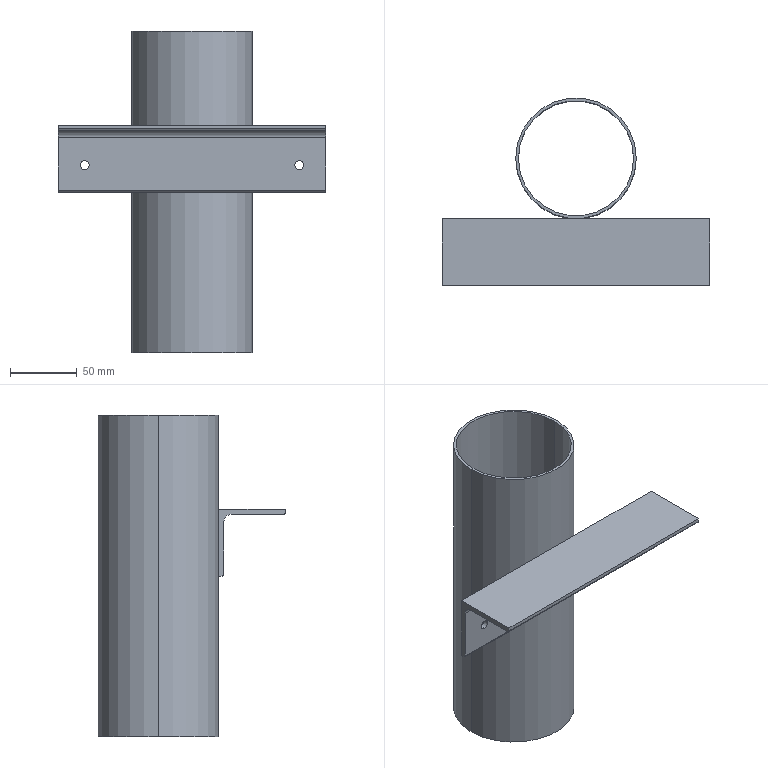Part | SolidWorks | features 3DProfileFeature 1, HoleWzd 1, ICE 1, WeldMemberFeat 1, WeldmentFeature 1 | 2 solids | 21 faces | box 200 x 140 x 240 mm | volume 210373 mm3 | cylinder 11 | plane 10 | commonest cylinder face diameters 6.6 x4 2.667 x2 86 x2 90 x2 11 x1
STEP:
#1=CARTESIAN_POINT('',(143.,45.,70.));
#2=VERTEX_POINT('',#1);
#3=CARTESIAN_POINT('',(57.,45.,70.));
#4=VERTEX_POINT('',#3);
#5=CARTESIAN_POINT('',(100.,45.,70.));
#6=DIRECTION('',(0.,0.,-1.));
#7=DIRECTION('',(-1.,0.,0.));
#8=AXIS2_PLACEMENT_3D('',#5,#6,#7);
#9=CIRCLE('',#8,43.);
#10=EDGE_CURVE('',#2,#4,#9,.T.);
#11=ORIENTED_EDGE('',*,*,#10,.F.);
#12=CARTESIAN_POINT('',(143.,45.,-170.));
#13=VERTEX_POINT('',#12);
#14=CARTESIAN_POINT('',(143.,45.,70.));
#15=DIRECTION('',(0.,0.,-1.));
#16=VECTOR('',#15,1000.);
#17=LINE('',#14,#16);
#18=EDGE_CURVE('',#2,#13,#17,.T.);
#19=ORIENTED_EDGE('',*,*,#18,.T.);
#20=CARTESIAN_POINT('',(57.,45.,-170.));
#21=VERTEX_POINT('',#20);
#22=CARTESIAN_POINT('',(100.,45.,-170.));
#23=DIRECTION('',(0.,0.,-1.));
#24=DIRECTION('',(-1.,0.,0.));
#25=AXIS2_PLACEMENT_3D('',#22,#23,#24);
#26=CIRCLE('',#25,43.);
#27=EDGE_CURVE('',#13,#21,#26,.T.);
#28=ORIENTED_EDGE('',*,*,#27,.T.);
#29=CARTESIAN_POINT('',(57.,45.,70.));
#30=DIRECTION('',(0.,0.,-1.));
#31=VECTOR('',#30,1000.);
#32=LINE('',#29,#31);
#33=EDGE_CURVE('',#4,#21,#32,.T.);
#34=ORIENTED_EDGE('',*,*,#33,.F.);
#35=EDGE_LOOP('',(#11,#19,#28,#34));
#36=FACE_OUTER_BOUND('',#35,.T.);
#37=CARTESIAN_POINT('',(100.,45.,70.));
#38=DIRECTION('',(0.,0.,-1.));
#39=DIRECTION('',(-1.,0.,0.));
#40=AXIS2_PLACEMENT_3D('',#37,#38,#39);
#41=CYLINDRICAL_SURFACE('',#40,43.);
#42=ADVANCED_FACE('',(#36),#41,.F.);
#43=CARTESIAN_POINT('',(55.,45.,70.));
#44=VERTEX_POINT('',#43);
#45=CARTESIAN_POINT('',(145.,45.,70.));
#46=VERTEX_POINT('',#45);
#47=CARTESIAN_POINT('',(100.,45.,70.));
#48=DIRECTION('',(0.,0.,-1.));
#49=DIRECTION('',(-1.,0.,0.));
#50=AXIS2_PLACEMENT_3D('',#47,#48,#49);
#51=CIRCLE('',#50,45.);
#52=EDGE_CURVE('',#44,#46,#51,.T.);
#53=ORIENTED_EDGE('',*,*,#52,.T.);
#54=CARTESIAN_POINT('',(145.,45.,-170.));
#55=VERTEX_POINT('',#54);
#56=CARTESIAN_POINT('',(145.,45.,70.));
#57=DIRECTION('',(0.,0.,-1.));
#58=VECTOR('',#57,1000.);
#59=LINE('',#56,#58);
#60=EDGE_CURVE('',#46,#55,#59,.T.);
#61=ORIENTED_EDGE('',*,*,#60,.T.);
#62=CARTESIAN_POINT('',(55.,45.,-170.));
#63=VERTEX_POINT('',#62);
#64=CARTESIAN_POINT('',(100.,45.,-170.));
#65=DIRECTION('',(0.,0.,-1.));
#66=DIRECTION('',(-1.,0.,0.));
#67=AXIS2_PLACEMENT_3D('',#64,#65,#66);
#68=CIRCLE('',#67,45.);
#69=EDGE_CURVE('',#63,#55,#68,.T.);
#70=ORIENTED_EDGE('',*,*,#69,.F.);
#71=CARTESIAN_POINT('',(55.,45.,70.));
#72=DIRECTION('',(0.,0.,-1.));
#73=VECTOR('',#72,1000.);
#74=LINE('',#71,#73);
#75=EDGE_CURVE('',#44,#63,#74,.T.);
#76=ORIENTED_EDGE('',*,*,#75,.F.);
#77=EDGE_LOOP('',(#53,#61,#70,#76));
#78=FACE_OUTER_BOUND('',#77,.T.);
#79=CARTESIAN_POINT('',(100.,45.,70.));
#80=DIRECTION('',(0.,0.,-1.));
#81=DIRECTION('',(-1.,0.,0.));
#82=AXIS2_PLACEMENT_3D('',#79,#80,#81);
#83=CYLINDRICAL_SURFACE('',#82,45.);
#84=ADVANCED_FACE('',(#78),#83,.T.);
#85=ORIENTED_EDGE('',*,*,#60,.F.);
#86=CARTESIAN_POINT('',(100.,45.,70.));
#87=DIRECTION('',(0.,0.,-1.));
#88=DIRECTION('',(-1.,0.,0.));
#89=AXIS2_PLACEMENT_3D('',#86,#87,#88);
#90=CIRCLE('',#89,45.);
#91=EDGE_CURVE('',#46,#44,#90,.T.);
#92=ORIENTED_EDGE('',*,*,#91,.T.);
#93=ORIENTED_EDGE('',*,*,#75,.T.);
#94=CARTESIAN_POINT('',(100.,45.,-170.));
#95=DIRECTION('',(0.,0.,-1.));
#96=DIRECTION('',(-1.,0.,0.));
#97=AXIS2_PLACEMENT_3D('',#94,#95,#96);
#98=CIRCLE('',#97,45.);
#99=EDGE_CURVE('',#55,#63,#98,.T.);
#100=ORIENTED_EDGE('',*,*,#99,.F.);
#101=EDGE_LOOP('',(#85,#92,#93,#100));
#102=FACE_OUTER_BOUND('',#101,.T.);
#103=CARTESIAN_POINT('',(100.,45.,70.));
#104=DIRECTION('',(0.,0.,-1.));
#105=DIRECTION('',(-1.,0.,0.));
#106=AXIS2_PLACEMENT_3D('',#103,#104,#105);
#107=CYLINDRICAL_SURFACE('',#106,45.);
#108=ADVANCED_FACE('',(#102),#107,.T.);
#109=CARTESIAN_POINT('',(100.,45.,70.));
#110=DIRECTION('',(0.,0.,-1.));
#111=DIRECTION('',(-1.,0.,0.));
#112=AXIS2_PLACEMENT_3D('',#109,#110,#111);
#113=CIRCLE('',#112,43.);
#114=EDGE_CURVE('',#4,#2,#113,.T.);
#115=ORIENTED_EDGE('',*,*,#114,.T.);
#116=ORIENTED_EDGE('',*,*,#10,.T.);
#117=EDGE_LOOP('',(#115,#116));
#118=FACE_BOUND('',#117,.T.);
#119=ORIENTED_EDGE('',*,*,#52,.F.);
#120=ORIENTED_EDGE('',*,*,#91,.F.);
#121=EDGE_LOOP('',(#119,#120));
#122=FACE_OUTER_BOUND('',#121,.T.);
#123=CARTESIAN_POINT('',(100.,45.,70.));
#124=DIRECTION('',(0.,0.,-1.));
#125=DIRECTION('',(-1.,0.,0.));
#126=AXIS2_PLACEMENT_3D('',#123,#124,#125);
#127=PLANE('',#126);
#128=ADVANCED_FACE('',(#118,#122),#127,.F.);
#129=CARTESIAN_POINT('',(100.,45.,-170.));
#130=DIRECTION('',(0.,0.,-1.));
#131=DIRECTION('',(-1.,0.,0.));
#132=AXIS2_PLACEMENT_3D('',#129,#130,#131);
#133=CIRCLE('',#132,43.);
#134=EDGE_CURVE('',#21,#13,#133,.T.);
#135=ORIENTED_EDGE('',*,*,#134,.F.);
#136=ORIENTED_EDGE('',*,*,#27,.F.);
#137=EDGE_LOOP('',(#135,#136));
#138=FACE_BOUND('',#137,.T.);
#139=ORIENTED_EDGE('',*,*,#69,.T.);
#140=ORIENTED_EDGE('',*,*,#99,.T.);
#141=EDGE_LOOP('',(#139,#140));
#142=FACE_OUTER_BOUND('',#141,.T.);
#143=CARTESIAN_POINT('',(100.,45.,-170.));
#144=DIRECTION('',(0.,0.,-1.));
#145=DIRECTION('',(-1.,0.,0.));
#146=AXIS2_PLACEMENT_3D('',#143,#144,#145);
#147=PLANE('',#146);
#148=ADVANCED_FACE('',(#138,#142),#147,.T.);
#149=ORIENTED_EDGE('',*,*,#18,.F.);
#150=ORIENTED_EDGE('',*,*,#114,.F.);
#151=ORIENTED_EDGE('',*,*,#33,.T.);
#152=ORIENTED_EDGE('',*,*,#134,.T.);
#153=EDGE_LOOP('',(#149,#150,#151,#152));
#154=FACE_OUTER_BOUND('',#153,.T.);
#155=CARTESIAN_POINT('',(100.,45.,70.));
#156=DIRECTION('',(0.,0.,-1.));
#157=DIRECTION('',(-1.,0.,0.));
#158=AXIS2_PLACEMENT_3D('',#155,#156,#157);
#159=CYLINDRICAL_SURFACE('',#158,43.);
#160=ADVANCED_FACE('',(#154),#159,.F.);
#161=CLOSED_SHELL('',(#42,#84,#108,#128,#148,#160));
#162=MANIFOLD_SOLID_BREP('',#161);
#163=CARTESIAN_POINT('',(20.,-4.,-33.3));
#164=VERTEX_POINT('',#163);
#165=CARTESIAN_POINT('',(20.,-4.,-26.7));
#166=VERTEX_POINT('',#165);
#167=CARTESIAN_POINT('',(20.,-4.,-30.));
#168=DIRECTION('',(0.,1.,0.));
#169=DIRECTION('',(0.,0.,1.));
#170=AXIS2_PLACEMENT_3D('',#167,#168,#169);
#171=CIRCLE('',#170,3.3);
#172=EDGE_CURVE('',#164,#166,#171,.T.);
#173=ORIENTED_EDGE('',*,*,#172,.F.);
#174=CARTESIAN_POINT('',(20.,0.,-33.3));
#175=VERTEX_POINT('',#174);
#176=CARTESIAN_POINT('',(20.,0.,-33.3));
#177=DIRECTION('',(0.,1.,0.));
#178=VECTOR('',#177,1000.);
#179=LINE('',#176,#178);
#180=EDGE_CURVE('',#164,#175,#179,.T.);
#181=ORIENTED_EDGE('',*,*,#180,.T.);
#182=CARTESIAN_POINT('',(20.,0.,-26.7));
#183=VERTEX_POINT('',#182);
#184=CARTESIAN_POINT('',(20.,0.,-30.));
#185=DIRECTION('',(0.,1.,0.));
#186=DIRECTION('',(0.,0.,1.));
#187=AXIS2_PLACEMENT_3D('',#184,#185,#186);
#188=CIRCLE('',#187,3.3);
#189=EDGE_CURVE('',#175,#183,#188,.T.);
#190=ORIENTED_EDGE('',*,*,#189,.T.);
#191=CARTESIAN_POINT('',(20.,0.,-26.7));
#192=DIRECTION('',(0.,1.,0.));
#193=VECTOR('',#192,1000.);
#194=LINE('',#191,#193);
#195=EDGE_CURVE('',#166,#183,#194,.T.);
#196=ORIENTED_EDGE('',*,*,#195,.F.);
#197=EDGE_LOOP('',(#173,#181,#190,#196));
#198=FACE_OUTER_BOUND('',#197,.T.);
#199=CARTESIAN_POINT('',(20.,0.,-30.));
#200=DIRECTION('',(0.,1.,0.));
#201=DIRECTION('',(0.,0.,1.));
#202=AXIS2_PLACEMENT_3D('',#199,#200,#201);
#203=CYLINDRICAL_SURFACE('',#202,3.3);
#204=ADVANCED_FACE('',(#198),#203,.F.);
#205=CARTESIAN_POINT('',(180.,-4.,-33.3));
#206=VERTEX_POINT('',#205);
#207=CARTESIAN_POINT('',(180.,-4.,-26.7));
#208=VERTEX_POINT('',#207);
#209=CARTESIAN_POINT('',(180.,-4.,-30.));
#210=DIRECTION('',(0.,1.,0.));
#211=DIRECTION('',(0.,0.,1.));
#212=AXIS2_PLACEMENT_3D('',#209,#210,#211);
#213=CIRCLE('',#212,3.3);
#214=EDGE_CURVE('',#206,#208,#213,.T.);
#215=ORIENTED_EDGE('',*,*,#214,.F.);
#216=CARTESIAN_POINT('',(180.,0.,-33.3));
#217=VERTEX_POINT('',#216);
#218=CARTESIAN_POINT('',(180.,0.,-33.3));
#219=DIRECTION('',(0.,1.,0.));
#220=VECTOR('',#219,1000.);
#221=LINE('',#218,#220);
#222=EDGE_CURVE('',#206,#217,#221,.T.);
#223=ORIENTED_EDGE('',*,*,#222,.T.);
#224=CARTESIAN_POINT('',(180.,0.,-26.7));
#225=VERTEX_POINT('',#224);
#226=CARTESIAN_POINT('',(180.,0.,-30.));
#227=DIRECTION('',(0.,1.,0.));
#228=DIRECTION('',(0.,0.,1.));
#229=AXIS2_PLACEMENT_3D('',#226,#227,#228);
#230=CIRCLE('',#229,3.3);
#231=EDGE_CURVE('',#217,#225,#230,.T.);
#232=ORIENTED_EDGE('',*,*,#231,.T.);
#233=CARTESIAN_POINT('',(180.,0.,-26.7));
#234=DIRECTION('',(0.,1.,0.));
#235=VECTOR('',#234,1000.);
#236=LINE('',#233,#235);
#237=EDGE_CURVE('',#208,#225,#236,.T.);
#238=ORIENTED_EDGE('',*,*,#237,.F.);
#239=EDGE_LOOP('',(#215,#223,#232,#238));
#240=FACE_OUTER_BOUND('',#239,.T.);
#241=CARTESIAN_POINT('',(180.,0.,-30.));
#242=DIRECTION('',(0.,1.,0.));
#243=DIRECTION('',(0.,0.,1.));
#244=AXIS2_PLACEMENT_3D('',#241,#242,#243);
#245=CYLINDRICAL_SURFACE('',#244,3.3);
#246=ADVANCED_FACE('',(#240),#245,.F.);
#247=CARTESIAN_POINT('',(0.,-2.667,-50.));
#248=VERTEX_POINT('',#247);
#249=CARTESIAN_POINT('',(0.,0.,-50.));
#250=VERTEX_POINT('',#249);
#251=CARTESIAN_POINT('',(0.,0.,-50.));
#252=DIRECTION('',(0.,1.,0.));
#253=VECTOR('',#252,1000.);
#254=LINE('',#251,#253);
#255=EDGE_CURVE('',#248,#250,#254,.T.);
#256=ORIENTED_EDGE('',*,*,#255,.T.);
#257=CARTESIAN_POINT('',(200.,0.,-50.));
#258=VERTEX_POINT('',#257);
#259=CARTESIAN_POINT('',(200.,0.,-50.));
#260=DIRECTION('',(-1.,0.,0.));
#261=VECTOR('',#260,1000.);
#262=LINE('',#259,#261);
#263=EDGE_CURVE('',#258,#250,#262,.T.);
#264=ORIENTED_EDGE('',*,*,#263,.F.);
#265=CARTESIAN_POINT('',(200.,-2.667,-50.));
#266=VERTEX_POINT('',#265);
#267=CARTESIAN_POINT('',(200.,0.,-50.));
#268=DIRECTION('',(0.,1.,0.));
#269=VECTOR('',#268,1000.);
#270=LINE('',#267,#269);
#271=EDGE_CURVE('',#266,#258,#270,.T.);
#272=ORIENTED_EDGE('',*,*,#271,.F.);
#273=CARTESIAN_POINT('',(200.,-2.667,-50.));
#274=DIRECTION('',(-1.,0.,0.));
#275=VECTOR('',#274,1000.);
#276=LINE('',#273,#275);
#277=EDGE_CURVE('',#266,#248,#276,.T.);
#278=ORIENTED_EDGE('',*,*,#277,.T.);
#279=EDGE_LOOP('',(#256,#264,#272,#278));
#280=FACE_OUTER_BOUND('',#279,.T.);
#281=CARTESIAN_POINT('',(200.,0.,-50.));
#282=DIRECTION('',(0.,0.,1.));
#283=DIRECTION('',(1.,0.,0.));
#284=AXIS2_PLACEMENT_3D('',#281,#282,#283);
#285=PLANE('',#284);
#286=ADVANCED_FACE('',(#280),#285,.F.);
#287=CARTESIAN_POINT('',(20.,0.,-30.));
#288=DIRECTION('',(0.,1.,0.));
#289=DIRECTION('',(0.,0.,1.));
#290=AXIS2_PLACEMENT_3D('',#287,#288,#289);
#291=CIRCLE('',#290,3.3);
#292=EDGE_CURVE('',#183,#175,#291,.T.);
#293=ORIENTED_EDGE('',*,*,#292,.F.);
#294=ORIENTED_EDGE('',*,*,#189,.F.);
#295=EDGE_LOOP('',(#293,#294));
#296=FACE_BOUND('',#295,.T.);
#297=CARTESIAN_POINT('',(180.,0.,-30.));
#298=DIRECTION('',(0.,1.,0.));
#299=DIRECTION('',(0.,0.,1.));
#300=AXIS2_PLACEMENT_3D('',#297,#298,#299);
#301=CIRCLE('',#300,3.3);
#302=EDGE_CURVE('',#225,#217,#301,.T.);
#303=ORIENTED_EDGE('',*,*,#302,.F.);
#304=ORIENTED_EDGE('',*,*,#231,.F.);
#305=EDGE_LOOP('',(#303,#304));
#306=FACE_BOUND('',#305,.T.);
#307=CARTESIAN_POINT('',(0.,0.,0.));
#308=VERTEX_POINT('',#307);
#309=CARTESIAN_POINT('',(0.,0.,-50.));
#310=DIRECTION('',(0.,0.,1.));
#311=VECTOR('',#310,1000.);
#312=LINE('',#309,#311);
#313=EDGE_CURVE('',#250,#308,#312,.T.);
#314=ORIENTED_EDGE('',*,*,#313,.T.);
#315=CARTESIAN_POINT('',(200.,0.,0.));
#316=VERTEX_POINT('',#315);
#317=CARTESIAN_POINT('',(200.,0.,0.));
#318=DIRECTION('',(-1.,0.,0.));
#319=VECTOR('',#318,1000.);
#320=LINE('',#317,#319);
#321=EDGE_CURVE('',#316,#308,#320,.T.);
#322=ORIENTED_EDGE('',*,*,#321,.F.);
#323=CARTESIAN_POINT('',(200.,0.,-50.));
#324=DIRECTION('',(0.,0.,1.));
#325=VECTOR('',#324,1000.);
#326=LINE('',#323,#325);
#327=EDGE_CURVE('',#258,#316,#326,.T.);
#328=ORIENTED_EDGE('',*,*,#327,.F.);
#329=ORIENTED_EDGE('',*,*,#263,.T.);
#330=EDGE_LOOP('',(#314,#322,#328,#329));
#331=FACE_OUTER_BOUND('',#330,.T.);
#332=CARTESIAN_POINT('',(200.,0.,-50.));
#333=DIRECTION('',(0.,-1.,0.));
#334=DIRECTION('',(0.,0.,-1.));
#335=AXIS2_PLACEMENT_3D('',#332,#333,#334);
#336=PLANE('',#335);
#337=ADVANCED_FACE('',(#296,#306,#331),#336,.F.);
#338=CARTESIAN_POINT('',(0.,-50.,0.));
#339=VERTEX_POINT('',#338);
#340=CARTESIAN_POINT('',(0.,0.,0.));
#341=DIRECTION('',(0.,-1.,0.));
#342=VECTOR('',#341,1000.);
#343=LINE('',#340,#342);
#344=EDGE_CURVE('',#308,#339,#343,.T.);
#345=ORIENTED_EDGE('',*,*,#344,.T.);
#346=CARTESIAN_POINT('',(200.,-50.,0.));
#347=VERTEX_POINT('',#346);
#348=CARTESIAN_POINT('',(200.,-50.,0.));
#349=DIRECTION('',(-1.,0.,0.));
#350=VECTOR('',#349,1000.);
#351=LINE('',#348,#350);
#352=EDGE_CURVE('',#347,#339,#351,.T.);
#353=ORIENTED_EDGE('',*,*,#352,.F.);
#354=CARTESIAN_POINT('',(200.,0.,0.));
#355=DIRECTION('',(0.,-1.,0.));
#356=VECTOR('',#355,1000.);
#357=LINE('',#354,#356);
#358=EDGE_CURVE('',#316,#347,#357,.T.);
#359=ORIENTED_EDGE('',*,*,#358,.F.);
#360=ORIENTED_EDGE('',*,*,#321,.T.);
#361=EDGE_LOOP('',(#345,#353,#359,#360));
#362=FACE_OUTER_BOUND('',#361,.T.);
#363=CARTESIAN_POINT('',(200.,0.,0.));
#364=DIRECTION('',(0.,0.,-1.));
#365=DIRECTION('',(0.,1.,0.));
#366=AXIS2_PLACEMENT_3D('',#363,#364,#365);
#367=PLANE('',#366);
#368=ADVANCED_FACE('',(#362),#367,.F.);
#369=CARTESIAN_POINT('',(0.,-50.,-2.667));
#370=VERTEX_POINT('',#369);
#371=CARTESIAN_POINT('',(0.,-50.,0.));
#372=DIRECTION('',(0.,0.,-1.));
#373=VECTOR('',#372,1000.);
#374=LINE('',#371,#373);
#375=EDGE_CURVE('',#339,#370,#374,.T.);
#376=ORIENTED_EDGE('',*,*,#375,.T.);
#377=CARTESIAN_POINT('',(200.,-50.,-2.667));
#378=VERTEX_POINT('',#377);
#379=CARTESIAN_POINT('',(200.,-50.,-2.667));
#380=DIRECTION('',(-1.,0.,0.));
#381=VECTOR('',#380,1000.);
#382=LINE('',#379,#381);
#383=EDGE_CURVE('',#378,#370,#382,.T.);
#384=ORIENTED_EDGE('',*,*,#383,.F.);
#385=CARTESIAN_POINT('',(200.,-50.,0.));
#386=DIRECTION('',(0.,0.,-1.));
#387=VECTOR('',#386,1000.);
#388=LINE('',#385,#387);
#389=EDGE_CURVE('',#347,#378,#388,.T.);
#390=ORIENTED_EDGE('',*,*,#389,.F.);
#391=ORIENTED_EDGE('',*,*,#352,.T.);
#392=EDGE_LOOP('',(#376,#384,#390,#391));
#393=FACE_OUTER_BOUND('',#392,.T.);
#394=CARTESIAN_POINT('',(200.,-50.,0.));
#395=DIRECTION('',(0.,1.,0.));
#396=DIRECTION('',(0.,0.,1.));
#397=AXIS2_PLACEMENT_3D('',#394,#395,#396);
#398=PLANE('',#397);
#399=ADVANCED_FACE('',(#393),#398,.F.);
#400=CARTESIAN_POINT('',(0.,-48.667,-4.));
#401=VERTEX_POINT('',#400);
#402=CARTESIAN_POINT('',(0.,-48.667,-2.667));
#403=DIRECTION('',(1.,0.,0.));
#404=DIRECTION('',(0.,0.,-1.));
#405=AXIS2_PLACEMENT_3D('',#402,#403,#404);
#406=CIRCLE('',#405,1.333);
#407=EDGE_CURVE('',#370,#401,#406,.T.);
#408=ORIENTED_EDGE('',*,*,#407,.T.);
#409=CARTESIAN_POINT('',(200.,-48.667,-4.));
#410=VERTEX_POINT('',#409);
#411=CARTESIAN_POINT('',(200.,-48.667,-4.));
#412=DIRECTION('',(-1.,0.,0.));
#413=VECTOR('',#412,1000.);
#414=LINE('',#411,#413);
#415=EDGE_CURVE('',#410,#401,#414,.T.);
#416=ORIENTED_EDGE('',*,*,#415,.F.);
#417=CARTESIAN_POINT('',(200.,-48.667,-2.667));
#418=DIRECTION('',(1.,0.,0.));
#419=DIRECTION('',(0.,0.,-1.));
#420=AXIS2_PLACEMENT_3D('',#417,#418,#419);
#421=CIRCLE('',#420,1.333);
#422=EDGE_CURVE('',#378,#410,#421,.T.);
#423=ORIENTED_EDGE('',*,*,#422,.F.);
#424=ORIENTED_EDGE('',*,*,#383,.T.);
#425=EDGE_LOOP('',(#408,#416,#423,#424));
#426=FACE_OUTER_BOUND('',#425,.T.);
#427=CARTESIAN_POINT('',(200.,-48.667,-2.667));
#428=DIRECTION('',(-1.,0.,0.));
#429=DIRECTION('',(0.,0.,1.));
#430=AXIS2_PLACEMENT_3D('',#427,#428,#429);
#431=CYLINDRICAL_SURFACE('',#430,1.333);
#432=ADVANCED_FACE('',(#426),#431,.T.);
#433=CARTESIAN_POINT('',(0.,-9.5,-4.));
#434=VERTEX_POINT('',#433);
#435=CARTESIAN_POINT('',(0.,-9.5,-4.));
#436=DIRECTION('',(0.,1.,0.));
#437=VECTOR('',#436,1000.);
#438=LINE('',#435,#437);
#439=EDGE_CURVE('',#401,#434,#438,.T.);
#440=ORIENTED_EDGE('',*,*,#439,.T.);
#441=CARTESIAN_POINT('',(200.,-9.5,-4.));
#442=VERTEX_POINT('',#441);
#443=CARTESIAN_POINT('',(200.,-9.5,-4.));
#444=DIRECTION('',(-1.,0.,0.));
#445=VECTOR('',#444,1000.);
#446=LINE('',#443,#445);
#447=EDGE_CURVE('',#442,#434,#446,.T.);
#448=ORIENTED_EDGE('',*,*,#447,.F.);
#449=CARTESIAN_POINT('',(200.,-9.5,-4.));
#450=DIRECTION('',(0.,1.,0.));
#451=VECTOR('',#450,1000.);
#452=LINE('',#449,#451);
#453=EDGE_CURVE('',#410,#442,#452,.T.);
#454=ORIENTED_EDGE('',*,*,#453,.F.);
#455=ORIENTED_EDGE('',*,*,#415,.T.);
#456=EDGE_LOOP('',(#440,#448,#454,#455));
#457=FACE_OUTER_BOUND('',#456,.T.);
#458=CARTESIAN_POINT('',(200.,-9.5,-4.));
#459=DIRECTION('',(0.,0.,1.));
#460=DIRECTION('',(0.,-1.,0.));
#461=AXIS2_PLACEMENT_3D('',#458,#459,#460);
#462=PLANE('',#461);
#463=ADVANCED_FACE('',(#457),#462,.F.);
#464=CARTESIAN_POINT('',(0.,-4.,-9.5));
#465=VERTEX_POINT('',#464);
#466=CARTESIAN_POINT('',(0.,-9.5,-9.5));
#467=DIRECTION('',(-1.,0.,0.));
#468=DIRECTION('',(0.,0.,-1.));
#469=AXIS2_PLACEMENT_3D('',#466,#467,#468);
#470=CIRCLE('',#469,5.5);
#471=EDGE_CURVE('',#434,#465,#470,.T.);
#472=ORIENTED_EDGE('',*,*,#471,.T.);
#473=CARTESIAN_POINT('',(200.,-4.,-9.5));
#474=VERTEX_POINT('',#473);
#475=CARTESIAN_POINT('',(200.,-4.,-9.5));
#476=DIRECTION('',(-1.,0.,0.));
#477=VECTOR('',#476,1000.);
#478=LINE('',#475,#477);
#479=EDGE_CURVE('',#474,#465,#478,.T.);
#480=ORIENTED_EDGE('',*,*,#479,.F.);
#481=CARTESIAN_POINT('',(200.,-9.5,-9.5));
#482=DIRECTION('',(-1.,0.,0.));
#483=DIRECTION('',(0.,0.,-1.));
#484=AXIS2_PLACEMENT_3D('',#481,#482,#483);
#485=CIRCLE('',#484,5.5);
#486=EDGE_CURVE('',#442,#474,#485,.T.);
#487=ORIENTED_EDGE('',*,*,#486,.F.);
#488=ORIENTED_EDGE('',*,*,#447,.T.);
#489=EDGE_LOOP('',(#472,#480,#487,#488));
#490=FACE_OUTER_BOUND('',#489,.T.);
#491=CARTESIAN_POINT('',(200.,-9.5,-9.5));
#492=DIRECTION('',(-1.,0.,0.));
#493=DIRECTION('',(0.,0.,1.));
#494=AXIS2_PLACEMENT_3D('',#491,#492,#493);
#495=CYLINDRICAL_SURFACE('',#494,5.5);
#496=ADVANCED_FACE('',(#490),#495,.F.);
#497=CARTESIAN_POINT('',(20.,-4.,-30.));
#498=DIRECTION('',(0.,1.,0.));
#499=DIRECTION('',(0.,0.,1.));
#500=AXIS2_PLACEMENT_3D('',#497,#498,#499);
#501=CIRCLE('',#500,3.3);
#502=EDGE_CURVE('',#166,#164,#501,.T.);
#503=ORIENTED_EDGE('',*,*,#502,.T.);
#504=ORIENTED_EDGE('',*,*,#172,.T.);
#505=EDGE_LOOP('',(#503,#504));
#506=FACE_BOUND('',#505,.T.);
#507=CARTESIAN_POINT('',(180.,-4.,-30.));
#508=DIRECTION('',(0.,1.,0.));
#509=DIRECTION('',(0.,0.,1.));
#510=AXIS2_PLACEMENT_3D('',#507,#508,#509);
#511=CIRCLE('',#510,3.3);
#512=EDGE_CURVE('',#208,#206,#511,.T.);
#513=ORIENTED_EDGE('',*,*,#512,.T.);
#514=ORIENTED_EDGE('',*,*,#214,.T.);
#515=EDGE_LOOP('',(#513,#514));
#516=FACE_BOUND('',#515,.T.);
#517=CARTESIAN_POINT('',(0.,-4.,-48.667));
#518=VERTEX_POINT('',#517);
#519=CARTESIAN_POINT('',(0.,-4.,-48.667));
#520=DIRECTION('',(0.,0.,-1.));
#521=VECTOR('',#520,1000.);
#522=LINE('',#519,#521);
#523=EDGE_CURVE('',#465,#518,#522,.T.);
#524=ORIENTED_EDGE('',*,*,#523,.T.);
#525=CARTESIAN_POINT('',(200.,-4.,-48.667));
#526=VERTEX_POINT('',#525);
#527=CARTESIAN_POINT('',(200.,-4.,-48.667));
#528=DIRECTION('',(-1.,0.,0.));
#529=VECTOR('',#528,1000.);
#530=LINE('',#527,#529);
#531=EDGE_CURVE('',#526,#518,#530,.T.);
#532=ORIENTED_EDGE('',*,*,#531,.F.);
#533=CARTESIAN_POINT('',(200.,-4.,-48.667));
#534=DIRECTION('',(0.,0.,-1.));
#535=VECTOR('',#534,1000.);
#536=LINE('',#533,#535);
#537=EDGE_CURVE('',#474,#526,#536,.T.);
#538=ORIENTED_EDGE('',*,*,#537,.F.);
#539=ORIENTED_EDGE('',*,*,#479,.T.);
#540=EDGE_LOOP('',(#524,#532,#538,#539));
#541=FACE_OUTER_BOUND('',#540,.T.);
#542=CARTESIAN_POINT('',(200.,-4.,-48.667));
#543=DIRECTION('',(0.,1.,0.));
#544=DIRECTION('',(0.,0.,1.));
#545=AXIS2_PLACEMENT_3D('',#542,#543,#544);
#546=PLANE('',#545);
#547=ADVANCED_FACE('',(#506,#516,#541),#546,.F.);
#548=CARTESIAN_POINT('',(0.,-2.667,-48.667));
#549=DIRECTION('',(1.,0.,0.));
#550=DIRECTION('',(0.,0.,1.));
#551=AXIS2_PLACEMENT_3D('',#548,#549,#550);
#552=CIRCLE('',#551,1.333);
#553=EDGE_CURVE('',#518,#248,#552,.T.);
#554=ORIENTED_EDGE('',*,*,#553,.T.);
#555=ORIENTED_EDGE('',*,*,#277,.F.);
#556=CARTESIAN_POINT('',(200.,-2.667,-48.667));
#557=DIRECTION('',(1.,0.,0.));
#558=DIRECTION('',(0.,0.,1.));
#559=AXIS2_PLACEMENT_3D('',#556,#557,#558);
#560=CIRCLE('',#559,1.333);
#561=EDGE_CURVE('',#526,#266,#560,.T.);
#562=ORIENTED_EDGE('',*,*,#561,.F.);
#563=ORIENTED_EDGE('',*,*,#531,.T.);
#564=EDGE_LOOP('',(#554,#555,#562,#563));
#565=FACE_OUTER_BOUND('',#564,.T.);
#566=CARTESIAN_POINT('',(200.,-2.667,-48.667));
#567=DIRECTION('',(-1.,0.,0.));
#568=DIRECTION('',(0.,0.,1.));
#569=AXIS2_PLACEMENT_3D('',#566,#567,#568);
#570=CYLINDRICAL_SURFACE('',#569,1.333);
#571=ADVANCED_FACE('',(#565),#570,.T.);
#572=ORIENTED_EDGE('',*,*,#271,.T.);
#573=ORIENTED_EDGE('',*,*,#327,.T.);
#574=ORIENTED_EDGE('',*,*,#358,.T.);
#575=ORIENTED_EDGE('',*,*,#389,.T.);
#576=ORIENTED_EDGE('',*,*,#422,.T.);
#577=ORIENTED_EDGE('',*,*,#453,.T.);
#578=ORIENTED_EDGE('',*,*,#486,.T.);
#579=ORIENTED_EDGE('',*,*,#537,.T.);
#580=ORIENTED_EDGE('',*,*,#561,.T.);
#581=EDGE_LOOP('',(#572,#573,#574,#575,#576,#577,#578,#579,#580));
#582=FACE_OUTER_BOUND('',#581,.T.);
#583=CARTESIAN_POINT('',(200.,-2.667,-48.667));
#584=DIRECTION('',(-1.,0.,0.));
#585=DIRECTION('',(0.,0.,1.));
#586=AXIS2_PLACEMENT_3D('',#583,#584,#585);
#587=PLANE('',#586);
#588=ADVANCED_FACE('',(#582),#587,.F.);
#589=ORIENTED_EDGE('',*,*,#255,.F.);
#590=ORIENTED_EDGE('',*,*,#553,.F.);
#591=ORIENTED_EDGE('',*,*,#523,.F.);
#592=ORIENTED_EDGE('',*,*,#471,.F.);
#593=ORIENTED_EDGE('',*,*,#439,.F.);
#594=ORIENTED_EDGE('',*,*,#407,.F.);
#595=ORIENTED_EDGE('',*,*,#375,.F.);
#596=ORIENTED_EDGE('',*,*,#344,.F.);
#597=ORIENTED_EDGE('',*,*,#313,.F.);
#598=EDGE_LOOP('',(#589,#590,#591,#592,#593,#594,#595,#596,#597));
#599=FACE_OUTER_BOUND('',#598,.T.);
#600=CARTESIAN_POINT('',(0.,-2.667,-48.667));
#601=DIRECTION('',(-1.,0.,0.));
#602=DIRECTION('',(0.,0.,1.));
#603=AXIS2_PLACEMENT_3D('',#600,#601,#602);
#604=PLANE('',#603);
#605=ADVANCED_FACE('',(#599),#604,.T.);
#606=ORIENTED_EDGE('',*,*,#222,.F.);
#607=ORIENTED_EDGE('',*,*,#512,.F.);
#608=ORIENTED_EDGE('',*,*,#237,.T.);
#609=ORIENTED_EDGE('',*,*,#302,.T.);
#610=EDGE_LOOP('',(#606,#607,#608,#609));
#611=FACE_OUTER_BOUND('',#610,.T.);
#612=CARTESIAN_POINT('',(180.,0.,-30.));
#613=DIRECTION('',(0.,1.,0.));
#614=DIRECTION('',(0.,0.,1.));
#615=AXIS2_PLACEMENT_3D('',#612,#613,#614);
#616=CYLINDRICAL_SURFACE('',#615,3.3);
#617=ADVANCED_FACE('',(#611),#616,.F.);
#618=ORIENTED_EDGE('',*,*,#180,.F.);
#619=ORIENTED_EDGE('',*,*,#502,.F.);
#620=ORIENTED_EDGE('',*,*,#195,.T.);
#621=ORIENTED_EDGE('',*,*,#292,.T.);
#622=EDGE_LOOP('',(#618,#619,#620,#621));
#623=FACE_OUTER_BOUND('',#622,.T.);
#624=CARTESIAN_POINT('',(20.,0.,-30.));
#625=DIRECTION('',(0.,1.,0.));
#626=DIRECTION('',(0.,0.,1.));
#627=AXIS2_PLACEMENT_3D('',#624,#625,#626);
#628=CYLINDRICAL_SURFACE('',#627,3.3);
#629=ADVANCED_FACE('',(#623),#628,.F.);
#630=CLOSED_SHELL('',(#204,#246,#286,#337,#368,#399,#432,#463,#496,#547,#571,#588,#605,#617,#629));
#631=MANIFOLD_SOLID_BREP('',#630);
#632=CARTESIAN_POINT('',(0.,0.,0.));
#633=DIRECTION('',(0.,0.,1.));
#634=DIRECTION('',(1.,0.,0.));
#635=AXIS2_PLACEMENT_3D('',#632,#633,#634);
#636=(LENGTH_UNIT()NAMED_UNIT(*)SI_UNIT(.MILLI.,.METRE.));
#637=UNCERTAINTY_MEASURE_WITH_UNIT(LENGTH_MEASURE(0.00001),#636,'','');
#638=(NAMED_UNIT(*)PLANE_ANGLE_UNIT()SI_UNIT($,.RADIAN.));
#639=(NAMED_UNIT(*)SI_UNIT($,.STERADIAN.)SOLID_ANGLE_UNIT());
#640=(GEOMETRIC_REPRESENTATION_CONTEXT(3)GLOBAL_UNCERTAINTY_ASSIGNED_CONTEXT((#637))GLOBAL_UNIT_ASSIGNED_CONTEXT((#636,#638,#639))REPRESENTATION_CONTEXT('',''));
#641=ADVANCED_BREP_SHAPE_REPRESENTATION('',(#162,#631,#635),#640);